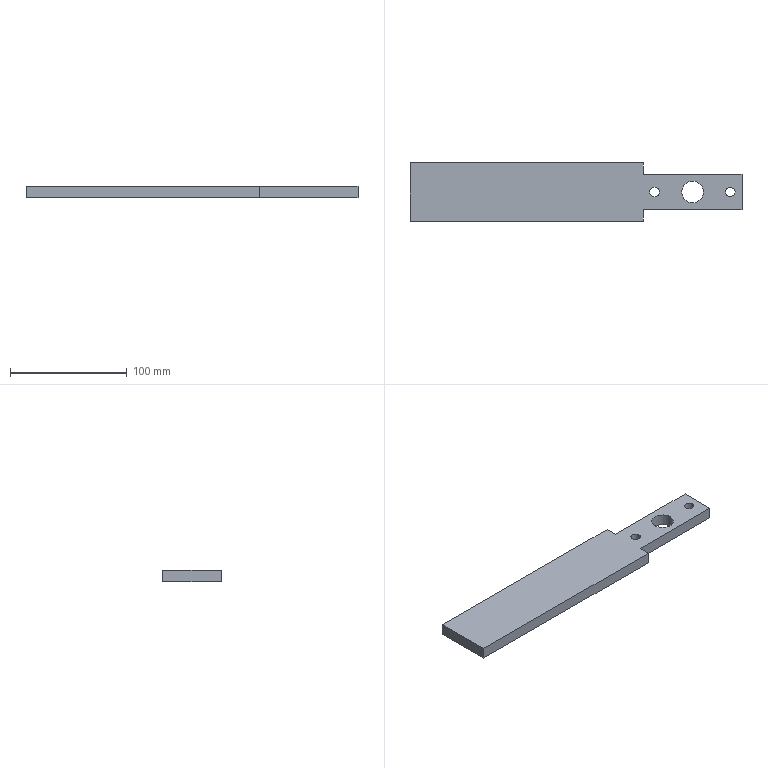Part | STEP file | Part 9^出料机械手-2 | 1 solid | 16 faces | box 284.646 x 50 x 10 mm | volume 121671 mm3 | plane 10 | cylinder 6 | commonest cylinder face diameters 8 x4 18.6 x2
STEP:
#1=CARTESIAN_POINT('',(59.477,0.,0.));
#2=VERTEX_POINT('',#1);
#3=CARTESIAN_POINT('',(40.877,0.,0.));
#4=VERTEX_POINT('',#3);
#5=CARTESIAN_POINT('',(50.177,0.,0.));
#6=DIRECTION('',(0.,0.,-1.));
#7=DIRECTION('',(-1.,0.,0.));
#8=AXIS2_PLACEMENT_3D('',#5,#6,#7);
#9=CIRCLE('',#8,9.3);
#10=EDGE_CURVE('',#2,#4,#9,.T.);
#11=ORIENTED_EDGE('',*,*,#10,.T.);
#12=CARTESIAN_POINT('',(40.877,0.,10.));
#13=VERTEX_POINT('',#12);
#14=CARTESIAN_POINT('',(40.877,0.,-2.));
#15=DIRECTION('',(0.,0.,1.));
#16=VECTOR('',#15,1000.);
#17=LINE('',#14,#16);
#18=EDGE_CURVE('',#4,#13,#17,.T.);
#19=ORIENTED_EDGE('',*,*,#18,.T.);
#20=CARTESIAN_POINT('',(59.477,0.,10.));
#21=VERTEX_POINT('',#20);
#22=CARTESIAN_POINT('',(50.177,0.,10.));
#23=DIRECTION('',(0.,0.,1.));
#24=DIRECTION('',(1.,0.,0.));
#25=AXIS2_PLACEMENT_3D('',#22,#23,#24);
#26=CIRCLE('',#25,9.3);
#27=EDGE_CURVE('',#13,#21,#26,.T.);
#28=ORIENTED_EDGE('',*,*,#27,.T.);
#29=CARTESIAN_POINT('',(59.477,0.,-2.));
#30=DIRECTION('',(0.,0.,1.));
#31=VECTOR('',#30,1000.);
#32=LINE('',#29,#31);
#33=EDGE_CURVE('',#2,#21,#32,.T.);
#34=ORIENTED_EDGE('',*,*,#33,.F.);
#35=EDGE_LOOP('',(#11,#19,#28,#34));
#36=FACE_OUTER_BOUND('',#35,.T.);
#37=CARTESIAN_POINT('',(50.177,0.,-2.));
#38=DIRECTION('',(0.,0.,1.));
#39=DIRECTION('',(1.,0.,0.));
#40=AXIS2_PLACEMENT_3D('',#37,#38,#39);
#41=CYLINDRICAL_SURFACE('',#40,9.3);
#42=ADVANCED_FACE('',(#36),#41,.F.);
#43=CARTESIAN_POINT('',(78.5,0.,10.));
#44=VERTEX_POINT('',#43);
#45=CARTESIAN_POINT('',(86.5,0.,10.));
#46=VERTEX_POINT('',#45);
#47=CARTESIAN_POINT('',(82.5,0.,10.));
#48=DIRECTION('',(0.,0.,1.));
#49=DIRECTION('',(1.,0.,0.));
#50=AXIS2_PLACEMENT_3D('',#47,#48,#49);
#51=CIRCLE('',#50,4.);
#52=EDGE_CURVE('',#44,#46,#51,.T.);
#53=ORIENTED_EDGE('',*,*,#52,.T.);
#54=CARTESIAN_POINT('',(86.5,0.,0.));
#55=VERTEX_POINT('',#54);
#56=CARTESIAN_POINT('',(86.5,0.,10.));
#57=DIRECTION('',(0.,0.,-1.));
#58=VECTOR('',#57,1000.);
#59=LINE('',#56,#58);
#60=EDGE_CURVE('',#46,#55,#59,.T.);
#61=ORIENTED_EDGE('',*,*,#60,.T.);
#62=CARTESIAN_POINT('',(78.5,0.,0.));
#63=VERTEX_POINT('',#62);
#64=CARTESIAN_POINT('',(82.5,0.,0.));
#65=DIRECTION('',(0.,0.,1.));
#66=DIRECTION('',(1.,0.,0.));
#67=AXIS2_PLACEMENT_3D('',#64,#65,#66);
#68=CIRCLE('',#67,4.);
#69=EDGE_CURVE('',#63,#55,#68,.T.);
#70=ORIENTED_EDGE('',*,*,#69,.F.);
#71=CARTESIAN_POINT('',(78.5,0.,10.));
#72=DIRECTION('',(0.,0.,-1.));
#73=VECTOR('',#72,1000.);
#74=LINE('',#71,#73);
#75=EDGE_CURVE('',#44,#63,#74,.T.);
#76=ORIENTED_EDGE('',*,*,#75,.F.);
#77=EDGE_LOOP('',(#53,#61,#70,#76));
#78=FACE_OUTER_BOUND('',#77,.T.);
#79=CARTESIAN_POINT('',(82.5,0.,10.));
#80=DIRECTION('',(0.,0.,-1.));
#81=DIRECTION('',(-1.,0.,0.));
#82=AXIS2_PLACEMENT_3D('',#79,#80,#81);
#83=CYLINDRICAL_SURFACE('',#82,4.);
#84=ADVANCED_FACE('',(#78),#83,.F.);
#85=CARTESIAN_POINT('',(13.5,0.,10.));
#86=VERTEX_POINT('',#85);
#87=CARTESIAN_POINT('',(21.5,0.,10.));
#88=VERTEX_POINT('',#87);
#89=CARTESIAN_POINT('',(17.5,0.,10.));
#90=DIRECTION('',(0.,0.,1.));
#91=DIRECTION('',(1.,0.,0.));
#92=AXIS2_PLACEMENT_3D('',#89,#90,#91);
#93=CIRCLE('',#92,4.);
#94=EDGE_CURVE('',#86,#88,#93,.T.);
#95=ORIENTED_EDGE('',*,*,#94,.T.);
#96=CARTESIAN_POINT('',(21.5,0.,0.));
#97=VERTEX_POINT('',#96);
#98=CARTESIAN_POINT('',(21.5,0.,10.));
#99=DIRECTION('',(0.,0.,-1.));
#100=VECTOR('',#99,1000.);
#101=LINE('',#98,#100);
#102=EDGE_CURVE('',#88,#97,#101,.T.);
#103=ORIENTED_EDGE('',*,*,#102,.T.);
#104=CARTESIAN_POINT('',(13.5,0.,0.));
#105=VERTEX_POINT('',#104);
#106=CARTESIAN_POINT('',(17.5,0.,0.));
#107=DIRECTION('',(0.,0.,1.));
#108=DIRECTION('',(1.,0.,0.));
#109=AXIS2_PLACEMENT_3D('',#106,#107,#108);
#110=CIRCLE('',#109,4.);
#111=EDGE_CURVE('',#105,#97,#110,.T.);
#112=ORIENTED_EDGE('',*,*,#111,.F.);
#113=CARTESIAN_POINT('',(13.5,0.,10.));
#114=DIRECTION('',(0.,0.,-1.));
#115=VECTOR('',#114,1000.);
#116=LINE('',#113,#115);
#117=EDGE_CURVE('',#86,#105,#116,.T.);
#118=ORIENTED_EDGE('',*,*,#117,.F.);
#119=EDGE_LOOP('',(#95,#103,#112,#118));
#120=FACE_OUTER_BOUND('',#119,.T.);
#121=CARTESIAN_POINT('',(17.5,0.,10.));
#122=DIRECTION('',(0.,0.,-1.));
#123=DIRECTION('',(-1.,0.,0.));
#124=AXIS2_PLACEMENT_3D('',#121,#122,#123);
#125=CYLINDRICAL_SURFACE('',#124,4.);
#126=ADVANCED_FACE('',(#120),#125,.F.);
#127=CARTESIAN_POINT('',(50.177,0.,10.));
#128=DIRECTION('',(0.,0.,1.));
#129=DIRECTION('',(1.,0.,0.));
#130=AXIS2_PLACEMENT_3D('',#127,#128,#129);
#131=CIRCLE('',#130,9.3);
#132=EDGE_CURVE('',#21,#13,#131,.T.);
#133=ORIENTED_EDGE('',*,*,#132,.F.);
#134=ORIENTED_EDGE('',*,*,#27,.F.);
#135=EDGE_LOOP('',(#133,#134));
#136=FACE_BOUND('',#135,.T.);
#137=ORIENTED_EDGE('',*,*,#94,.F.);
#138=CARTESIAN_POINT('',(17.5,0.,10.));
#139=DIRECTION('',(0.,0.,1.));
#140=DIRECTION('',(1.,0.,0.));
#141=AXIS2_PLACEMENT_3D('',#138,#139,#140);
#142=CIRCLE('',#141,4.);
#143=EDGE_CURVE('',#88,#86,#142,.T.);
#144=ORIENTED_EDGE('',*,*,#143,.F.);
#145=EDGE_LOOP('',(#137,#144));
#146=FACE_BOUND('',#145,.T.);
#147=CARTESIAN_POINT('',(92.5,15.,10.));
#148=VERTEX_POINT('',#147);
#149=CARTESIAN_POINT('',(7.854,15.,10.));
#150=VERTEX_POINT('',#149);
#151=CARTESIAN_POINT('',(7.5,15.,10.));
#152=DIRECTION('',(-1.,0.,0.));
#153=VECTOR('',#152,1000.);
#154=LINE('',#151,#153);
#155=EDGE_CURVE('',#148,#150,#154,.T.);
#156=ORIENTED_EDGE('',*,*,#155,.T.);
#157=CARTESIAN_POINT('',(7.854,25.,10.));
#158=VERTEX_POINT('',#157);
#159=CARTESIAN_POINT('',(7.854,25.,10.));
#160=DIRECTION('',(0.,1.,0.));
#161=VECTOR('',#160,1000.);
#162=LINE('',#159,#161);
#163=EDGE_CURVE('',#150,#158,#162,.T.);
#164=ORIENTED_EDGE('',*,*,#163,.T.);
#165=CARTESIAN_POINT('',(-192.146,25.,10.));
#166=VERTEX_POINT('',#165);
#167=CARTESIAN_POINT('',(-192.146,25.,10.));
#168=DIRECTION('',(-1.,0.,0.));
#169=VECTOR('',#168,1000.);
#170=LINE('',#167,#169);
#171=EDGE_CURVE('',#158,#166,#170,.T.);
#172=ORIENTED_EDGE('',*,*,#171,.T.);
#173=CARTESIAN_POINT('',(-192.146,-25.,10.));
#174=VERTEX_POINT('',#173);
#175=CARTESIAN_POINT('',(-192.146,25.,10.));
#176=DIRECTION('',(0.,-1.,0.));
#177=VECTOR('',#176,1000.);
#178=LINE('',#175,#177);
#179=EDGE_CURVE('',#166,#174,#178,.T.);
#180=ORIENTED_EDGE('',*,*,#179,.T.);
#181=CARTESIAN_POINT('',(7.854,-25.,10.));
#182=VERTEX_POINT('',#181);
#183=CARTESIAN_POINT('',(-192.146,-25.,10.));
#184=DIRECTION('',(1.,0.,0.));
#185=VECTOR('',#184,1000.);
#186=LINE('',#183,#185);
#187=EDGE_CURVE('',#174,#182,#186,.T.);
#188=ORIENTED_EDGE('',*,*,#187,.T.);
#189=CARTESIAN_POINT('',(7.854,-15.,10.));
#190=VERTEX_POINT('',#189);
#191=CARTESIAN_POINT('',(7.854,25.,10.));
#192=DIRECTION('',(0.,1.,0.));
#193=VECTOR('',#192,1000.);
#194=LINE('',#191,#193);
#195=EDGE_CURVE('',#182,#190,#194,.T.);
#196=ORIENTED_EDGE('',*,*,#195,.T.);
#197=CARTESIAN_POINT('',(92.5,-15.,10.));
#198=VERTEX_POINT('',#197);
#199=CARTESIAN_POINT('',(7.5,-15.,10.));
#200=DIRECTION('',(1.,0.,0.));
#201=VECTOR('',#200,1000.);
#202=LINE('',#199,#201);
#203=EDGE_CURVE('',#190,#198,#202,.T.);
#204=ORIENTED_EDGE('',*,*,#203,.T.);
#205=CARTESIAN_POINT('',(92.5,-15.,10.));
#206=DIRECTION('',(0.,1.,0.));
#207=VECTOR('',#206,1000.);
#208=LINE('',#205,#207);
#209=EDGE_CURVE('',#198,#148,#208,.T.);
#210=ORIENTED_EDGE('',*,*,#209,.T.);
#211=EDGE_LOOP('',(#156,#164,#172,#180,#188,#196,#204,#210));
#212=FACE_OUTER_BOUND('',#211,.T.);
#213=ORIENTED_EDGE('',*,*,#52,.F.);
#214=CARTESIAN_POINT('',(82.5,0.,10.));
#215=DIRECTION('',(0.,0.,1.));
#216=DIRECTION('',(1.,0.,0.));
#217=AXIS2_PLACEMENT_3D('',#214,#215,#216);
#218=CIRCLE('',#217,4.);
#219=EDGE_CURVE('',#46,#44,#218,.T.);
#220=ORIENTED_EDGE('',*,*,#219,.F.);
#221=EDGE_LOOP('',(#213,#220));
#222=FACE_BOUND('',#221,.T.);
#223=CARTESIAN_POINT('',(92.5,15.,10.));
#224=DIRECTION('',(0.,0.,-1.));
#225=DIRECTION('',(-1.,0.,0.));
#226=AXIS2_PLACEMENT_3D('',#223,#224,#225);
#227=PLANE('',#226);
#228=ADVANCED_FACE('',(#136,#146,#212,#222),#227,.F.);
#229=ORIENTED_EDGE('',*,*,#10,.F.);
#230=CARTESIAN_POINT('',(50.177,0.,0.));
#231=DIRECTION('',(0.,0.,-1.));
#232=DIRECTION('',(-1.,0.,0.));
#233=AXIS2_PLACEMENT_3D('',#230,#231,#232);
#234=CIRCLE('',#233,9.3);
#235=EDGE_CURVE('',#4,#2,#234,.T.);
#236=ORIENTED_EDGE('',*,*,#235,.F.);
#237=EDGE_LOOP('',(#229,#236));
#238=FACE_BOUND('',#237,.T.);
#239=CARTESIAN_POINT('',(7.854,-15.,0.));
#240=VERTEX_POINT('',#239);
#241=CARTESIAN_POINT('',(92.5,-15.,0.));
#242=VERTEX_POINT('',#241);
#243=CARTESIAN_POINT('',(7.5,-15.,0.));
#244=DIRECTION('',(1.,0.,0.));
#245=VECTOR('',#244,1000.);
#246=LINE('',#243,#245);
#247=EDGE_CURVE('',#240,#242,#246,.T.);
#248=ORIENTED_EDGE('',*,*,#247,.F.);
#249=CARTESIAN_POINT('',(7.854,-25.,0.));
#250=VERTEX_POINT('',#249);
#251=CARTESIAN_POINT('',(7.854,25.,0.));
#252=DIRECTION('',(0.,1.,0.));
#253=VECTOR('',#252,1000.);
#254=LINE('',#251,#253);
#255=EDGE_CURVE('',#250,#240,#254,.T.);
#256=ORIENTED_EDGE('',*,*,#255,.F.);
#257=CARTESIAN_POINT('',(-192.146,-25.,0.));
#258=VERTEX_POINT('',#257);
#259=CARTESIAN_POINT('',(-192.146,-25.,0.));
#260=DIRECTION('',(1.,0.,0.));
#261=VECTOR('',#260,1000.);
#262=LINE('',#259,#261);
#263=EDGE_CURVE('',#258,#250,#262,.T.);
#264=ORIENTED_EDGE('',*,*,#263,.F.);
#265=CARTESIAN_POINT('',(-192.146,25.,0.));
#266=VERTEX_POINT('',#265);
#267=CARTESIAN_POINT('',(-192.146,25.,0.));
#268=DIRECTION('',(0.,-1.,0.));
#269=VECTOR('',#268,1000.);
#270=LINE('',#267,#269);
#271=EDGE_CURVE('',#266,#258,#270,.T.);
#272=ORIENTED_EDGE('',*,*,#271,.F.);
#273=CARTESIAN_POINT('',(7.854,25.,0.));
#274=VERTEX_POINT('',#273);
#275=CARTESIAN_POINT('',(-192.146,25.,0.));
#276=DIRECTION('',(-1.,0.,0.));
#277=VECTOR('',#276,1000.);
#278=LINE('',#275,#277);
#279=EDGE_CURVE('',#274,#266,#278,.T.);
#280=ORIENTED_EDGE('',*,*,#279,.F.);
#281=CARTESIAN_POINT('',(7.854,15.,0.));
#282=VERTEX_POINT('',#281);
#283=CARTESIAN_POINT('',(7.854,25.,0.));
#284=DIRECTION('',(0.,1.,0.));
#285=VECTOR('',#284,1000.);
#286=LINE('',#283,#285);
#287=EDGE_CURVE('',#282,#274,#286,.T.);
#288=ORIENTED_EDGE('',*,*,#287,.F.);
#289=CARTESIAN_POINT('',(92.5,15.,0.));
#290=VERTEX_POINT('',#289);
#291=CARTESIAN_POINT('',(7.5,15.,0.));
#292=DIRECTION('',(-1.,0.,0.));
#293=VECTOR('',#292,1000.);
#294=LINE('',#291,#293);
#295=EDGE_CURVE('',#290,#282,#294,.T.);
#296=ORIENTED_EDGE('',*,*,#295,.F.);
#297=CARTESIAN_POINT('',(92.5,-15.,0.));
#298=DIRECTION('',(0.,1.,0.));
#299=VECTOR('',#298,1000.);
#300=LINE('',#297,#299);
#301=EDGE_CURVE('',#242,#290,#300,.T.);
#302=ORIENTED_EDGE('',*,*,#301,.F.);
#303=EDGE_LOOP('',(#248,#256,#264,#272,#280,#288,#296,#302));
#304=FACE_OUTER_BOUND('',#303,.T.);
#305=ORIENTED_EDGE('',*,*,#111,.T.);
#306=CARTESIAN_POINT('',(17.5,0.,0.));
#307=DIRECTION('',(0.,0.,1.));
#308=DIRECTION('',(1.,0.,0.));
#309=AXIS2_PLACEMENT_3D('',#306,#307,#308);
#310=CIRCLE('',#309,4.);
#311=EDGE_CURVE('',#97,#105,#310,.T.);
#312=ORIENTED_EDGE('',*,*,#311,.T.);
#313=EDGE_LOOP('',(#305,#312));
#314=FACE_BOUND('',#313,.T.);
#315=ORIENTED_EDGE('',*,*,#69,.T.);
#316=CARTESIAN_POINT('',(82.5,0.,0.));
#317=DIRECTION('',(0.,0.,1.));
#318=DIRECTION('',(1.,0.,0.));
#319=AXIS2_PLACEMENT_3D('',#316,#317,#318);
#320=CIRCLE('',#319,4.);
#321=EDGE_CURVE('',#55,#63,#320,.T.);
#322=ORIENTED_EDGE('',*,*,#321,.T.);
#323=EDGE_LOOP('',(#315,#322));
#324=FACE_BOUND('',#323,.T.);
#325=CARTESIAN_POINT('',(92.5,15.,0.));
#326=DIRECTION('',(0.,0.,-1.));
#327=DIRECTION('',(-1.,0.,0.));
#328=AXIS2_PLACEMENT_3D('',#325,#326,#327);
#329=PLANE('',#328);
#330=ADVANCED_FACE('',(#238,#304,#314,#324),#329,.T.);
#331=ORIENTED_EDGE('',*,*,#301,.T.);
#332=CARTESIAN_POINT('',(92.5,15.,10.));
#333=DIRECTION('',(0.,0.,-1.));
#334=VECTOR('',#333,1000.);
#335=LINE('',#332,#334);
#336=EDGE_CURVE('',#148,#290,#335,.T.);
#337=ORIENTED_EDGE('',*,*,#336,.F.);
#338=ORIENTED_EDGE('',*,*,#209,.F.);
#339=CARTESIAN_POINT('',(92.5,-15.,10.));
#340=DIRECTION('',(0.,0.,-1.));
#341=VECTOR('',#340,1000.);
#342=LINE('',#339,#341);
#343=EDGE_CURVE('',#198,#242,#342,.T.);
#344=ORIENTED_EDGE('',*,*,#343,.T.);
#345=EDGE_LOOP('',(#331,#337,#338,#344));
#346=FACE_OUTER_BOUND('',#345,.T.);
#347=CARTESIAN_POINT('',(92.5,-15.,10.));
#348=DIRECTION('',(-1.,0.,0.));
#349=DIRECTION('',(0.,0.,1.));
#350=AXIS2_PLACEMENT_3D('',#347,#348,#349);
#351=PLANE('',#350);
#352=ADVANCED_FACE('',(#346),#351,.F.);
#353=ORIENTED_EDGE('',*,*,#295,.T.);
#354=CARTESIAN_POINT('',(7.854,15.,10.));
#355=DIRECTION('',(0.,0.,1.));
#356=VECTOR('',#355,1000.);
#357=LINE('',#354,#356);
#358=EDGE_CURVE('',#282,#150,#357,.T.);
#359=ORIENTED_EDGE('',*,*,#358,.T.);
#360=ORIENTED_EDGE('',*,*,#155,.F.);
#361=ORIENTED_EDGE('',*,*,#336,.T.);
#362=EDGE_LOOP('',(#353,#359,#360,#361));
#363=FACE_OUTER_BOUND('',#362,.T.);
#364=CARTESIAN_POINT('',(7.5,15.,10.));
#365=DIRECTION('',(0.,-1.,0.));
#366=DIRECTION('',(0.,0.,-1.));
#367=AXIS2_PLACEMENT_3D('',#364,#365,#366);
#368=PLANE('',#367);
#369=ADVANCED_FACE('',(#363),#368,.F.);
#370=ORIENTED_EDGE('',*,*,#203,.F.);
#371=CARTESIAN_POINT('',(7.854,-15.,10.));
#372=DIRECTION('',(0.,0.,-1.));
#373=VECTOR('',#372,1000.);
#374=LINE('',#371,#373);
#375=EDGE_CURVE('',#190,#240,#374,.T.);
#376=ORIENTED_EDGE('',*,*,#375,.T.);
#377=ORIENTED_EDGE('',*,*,#247,.T.);
#378=ORIENTED_EDGE('',*,*,#343,.F.);
#379=EDGE_LOOP('',(#370,#376,#377,#378));
#380=FACE_OUTER_BOUND('',#379,.T.);
#381=CARTESIAN_POINT('',(7.5,-15.,10.));
#382=DIRECTION('',(0.,1.,0.));
#383=DIRECTION('',(0.,0.,1.));
#384=AXIS2_PLACEMENT_3D('',#381,#382,#383);
#385=PLANE('',#384);
#386=ADVANCED_FACE('',(#380),#385,.F.);
#387=ORIENTED_EDGE('',*,*,#102,.F.);
#388=ORIENTED_EDGE('',*,*,#143,.T.);
#389=ORIENTED_EDGE('',*,*,#117,.T.);
#390=ORIENTED_EDGE('',*,*,#311,.F.);
#391=EDGE_LOOP('',(#387,#388,#389,#390));
#392=FACE_OUTER_BOUND('',#391,.T.);
#393=CARTESIAN_POINT('',(17.5,0.,10.));
#394=DIRECTION('',(0.,0.,-1.));
#395=DIRECTION('',(-1.,0.,0.));
#396=AXIS2_PLACEMENT_3D('',#393,#394,#395);
#397=CYLINDRICAL_SURFACE('',#396,4.);
#398=ADVANCED_FACE('',(#392),#397,.F.);
#399=ORIENTED_EDGE('',*,*,#60,.F.);
#400=ORIENTED_EDGE('',*,*,#219,.T.);
#401=ORIENTED_EDGE('',*,*,#75,.T.);
#402=ORIENTED_EDGE('',*,*,#321,.F.);
#403=EDGE_LOOP('',(#399,#400,#401,#402));
#404=FACE_OUTER_BOUND('',#403,.T.);
#405=CARTESIAN_POINT('',(82.5,0.,10.));
#406=DIRECTION('',(0.,0.,-1.));
#407=DIRECTION('',(-1.,0.,0.));
#408=AXIS2_PLACEMENT_3D('',#405,#406,#407);
#409=CYLINDRICAL_SURFACE('',#408,4.);
#410=ADVANCED_FACE('',(#404),#409,.F.);
#411=ORIENTED_EDGE('',*,*,#358,.F.);
#412=ORIENTED_EDGE('',*,*,#287,.T.);
#413=CARTESIAN_POINT('',(7.854,25.,0.));
#414=DIRECTION('',(0.,0.,1.));
#415=VECTOR('',#414,1000.);
#416=LINE('',#413,#415);
#417=EDGE_CURVE('',#274,#158,#416,.T.);
#418=ORIENTED_EDGE('',*,*,#417,.T.);
#419=ORIENTED_EDGE('',*,*,#163,.F.);
#420=EDGE_LOOP('',(#411,#412,#418,#419));
#421=FACE_OUTER_BOUND('',#420,.T.);
#422=CARTESIAN_POINT('',(7.854,25.,0.));
#423=DIRECTION('',(1.,0.,0.));
#424=DIRECTION('',(0.,1.,0.));
#425=AXIS2_PLACEMENT_3D('',#422,#423,#424);
#426=PLANE('',#425);
#427=ADVANCED_FACE('',(#421),#426,.T.);
#428=ORIENTED_EDGE('',*,*,#375,.F.);
#429=ORIENTED_EDGE('',*,*,#195,.F.);
#430=CARTESIAN_POINT('',(7.854,-25.,0.));
#431=DIRECTION('',(0.,0.,1.));
#432=VECTOR('',#431,1000.);
#433=LINE('',#430,#432);
#434=EDGE_CURVE('',#250,#182,#433,.T.);
#435=ORIENTED_EDGE('',*,*,#434,.F.);
#436=ORIENTED_EDGE('',*,*,#255,.T.);
#437=EDGE_LOOP('',(#428,#429,#435,#436));
#438=FACE_OUTER_BOUND('',#437,.T.);
#439=CARTESIAN_POINT('',(7.854,25.,0.));
#440=DIRECTION('',(1.,0.,0.));
#441=DIRECTION('',(0.,1.,0.));
#442=AXIS2_PLACEMENT_3D('',#439,#440,#441);
#443=PLANE('',#442);
#444=ADVANCED_FACE('',(#438),#443,.T.);
#445=ORIENTED_EDGE('',*,*,#187,.F.);
#446=CARTESIAN_POINT('',(-192.146,-25.,0.));
#447=DIRECTION('',(0.,0.,1.));
#448=VECTOR('',#447,1000.);
#449=LINE('',#446,#448);
#450=EDGE_CURVE('',#258,#174,#449,.T.);
#451=ORIENTED_EDGE('',*,*,#450,.F.);
#452=ORIENTED_EDGE('',*,*,#263,.T.);
#453=ORIENTED_EDGE('',*,*,#434,.T.);
#454=EDGE_LOOP('',(#445,#451,#452,#453));
#455=FACE_OUTER_BOUND('',#454,.T.);
#456=CARTESIAN_POINT('',(-192.146,-25.,0.));
#457=DIRECTION('',(0.,-1.,0.));
#458=DIRECTION('',(0.,0.,-1.));
#459=AXIS2_PLACEMENT_3D('',#456,#457,#458);
#460=PLANE('',#459);
#461=ADVANCED_FACE('',(#455),#460,.T.);
#462=ORIENTED_EDGE('',*,*,#179,.F.);
#463=CARTESIAN_POINT('',(-192.146,25.,0.));
#464=DIRECTION('',(0.,0.,1.));
#465=VECTOR('',#464,1000.);
#466=LINE('',#463,#465);
#467=EDGE_CURVE('',#266,#166,#466,.T.);
#468=ORIENTED_EDGE('',*,*,#467,.F.);
#469=ORIENTED_EDGE('',*,*,#271,.T.);
#470=ORIENTED_EDGE('',*,*,#450,.T.);
#471=EDGE_LOOP('',(#462,#468,#469,#470));
#472=FACE_OUTER_BOUND('',#471,.T.);
#473=CARTESIAN_POINT('',(-192.146,25.,0.));
#474=DIRECTION('',(-1.,0.,0.));
#475=DIRECTION('',(0.,0.,1.));
#476=AXIS2_PLACEMENT_3D('',#473,#474,#475);
#477=PLANE('',#476);
#478=ADVANCED_FACE('',(#472),#477,.T.);
#479=ORIENTED_EDGE('',*,*,#171,.F.);
#480=ORIENTED_EDGE('',*,*,#417,.F.);
#481=ORIENTED_EDGE('',*,*,#279,.T.);
#482=ORIENTED_EDGE('',*,*,#467,.T.);
#483=EDGE_LOOP('',(#479,#480,#481,#482));
#484=FACE_OUTER_BOUND('',#483,.T.);
#485=CARTESIAN_POINT('',(-192.146,25.,0.));
#486=DIRECTION('',(0.,1.,0.));
#487=DIRECTION('',(0.,0.,1.));
#488=AXIS2_PLACEMENT_3D('',#485,#486,#487);
#489=PLANE('',#488);
#490=ADVANCED_FACE('',(#484),#489,.T.);
#491=ORIENTED_EDGE('',*,*,#18,.F.);
#492=ORIENTED_EDGE('',*,*,#235,.T.);
#493=ORIENTED_EDGE('',*,*,#33,.T.);
#494=ORIENTED_EDGE('',*,*,#132,.T.);
#495=EDGE_LOOP('',(#491,#492,#493,#494));
#496=FACE_OUTER_BOUND('',#495,.T.);
#497=CARTESIAN_POINT('',(50.177,0.,-2.));
#498=DIRECTION('',(0.,0.,1.));
#499=DIRECTION('',(1.,0.,0.));
#500=AXIS2_PLACEMENT_3D('',#497,#498,#499);
#501=CYLINDRICAL_SURFACE('',#500,9.3);
#502=ADVANCED_FACE('',(#496),#501,.F.);
#503=CLOSED_SHELL('',(#42,#84,#126,#228,#330,#352,#369,#386,#398,#410,#427,#444,#461,#478,#490,#502));
#504=MANIFOLD_SOLID_BREP('',#503);
#505=CARTESIAN_POINT('',(0.,0.,0.));
#506=DIRECTION('',(0.,0.,1.));
#507=DIRECTION('',(1.,0.,0.));
#508=AXIS2_PLACEMENT_3D('',#505,#506,#507);
#509=(LENGTH_UNIT()NAMED_UNIT(*)SI_UNIT(.MILLI.,.METRE.));
#510=UNCERTAINTY_MEASURE_WITH_UNIT(LENGTH_MEASURE(0.00001),#509,'','');
#511=(NAMED_UNIT(*)PLANE_ANGLE_UNIT()SI_UNIT($,.RADIAN.));
#512=(NAMED_UNIT(*)SI_UNIT($,.STERADIAN.)SOLID_ANGLE_UNIT());
#513=(GEOMETRIC_REPRESENTATION_CONTEXT(3)GLOBAL_UNCERTAINTY_ASSIGNED_CONTEXT((#510))GLOBAL_UNIT_ASSIGNED_CONTEXT((#509,#511,#512))REPRESENTATION_CONTEXT('',''));
#514=ADVANCED_BREP_SHAPE_REPRESENTATION('',(#504,#508),#513);